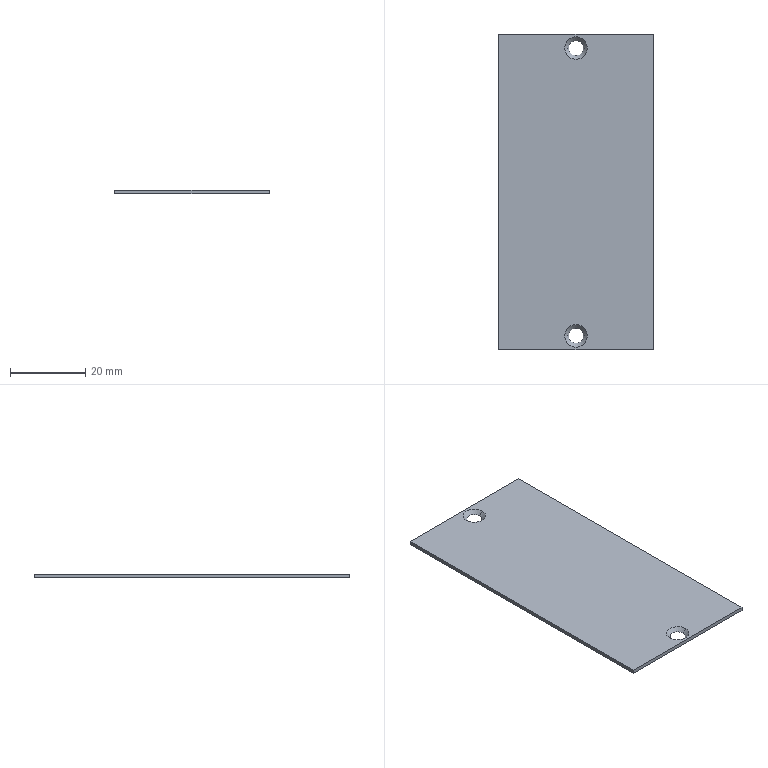Part | SolidWorks | features BaseBody 1 | 1 solid | 10 faces | box 41 x 84 x 1 mm | volume 3404 mm3 | plane 6 | cone 4
STEP:
#1=CARTESIAN_POINT('',(2.,-38.3,0.));
#2=VERTEX_POINT('',#1);
#3=CARTESIAN_POINT('',(-2.,-38.3,0.));
#4=VERTEX_POINT('',#3);
#5=CARTESIAN_POINT('',(0.,-38.3,0.));
#6=DIRECTION('',(0.,0.,-1.));
#7=DIRECTION('',(1.,0.,0.));
#8=AXIS2_PLACEMENT_3D('',#5,#6,#7);
#9=CIRCLE('',#8,2.);
#10=EDGE_CURVE('',#2,#4,#9,.T.);
#11=ORIENTED_EDGE('',*,*,#10,.T.);
#12=CARTESIAN_POINT('',(-3.,-38.3,1.));
#13=VERTEX_POINT('',#12);
#14=CARTESIAN_POINT('',(-3.,-38.3,1.));
#15=DIRECTION('',(-0.7071,0.,0.7071));
#16=VECTOR('',#15,1000.);
#17=LINE('',#14,#16);
#18=EDGE_CURVE('',#4,#13,#17,.T.);
#19=ORIENTED_EDGE('',*,*,#18,.T.);
#20=CARTESIAN_POINT('',(3.,-38.3,1.));
#21=VERTEX_POINT('',#20);
#22=CARTESIAN_POINT('',(0.,-38.3,1.));
#23=DIRECTION('',(0.,0.,-1.));
#24=DIRECTION('',(1.,0.,0.));
#25=AXIS2_PLACEMENT_3D('',#22,#23,#24);
#26=CIRCLE('',#25,3.);
#27=EDGE_CURVE('',#21,#13,#26,.T.);
#28=ORIENTED_EDGE('',*,*,#27,.F.);
#29=CARTESIAN_POINT('',(3.,-38.3,1.));
#30=DIRECTION('',(0.7071,0.,0.7071));
#31=VECTOR('',#30,1000.);
#32=LINE('',#29,#31);
#33=EDGE_CURVE('',#2,#21,#32,.T.);
#34=ORIENTED_EDGE('',*,*,#33,.F.);
#35=EDGE_LOOP('',(#11,#19,#28,#34));
#36=FACE_OUTER_BOUND('',#35,.T.);
#37=CARTESIAN_POINT('',(0.,-38.3,1.));
#38=DIRECTION('',(0.,0.,1.));
#39=DIRECTION('',(1.,0.,0.));
#40=AXIS2_PLACEMENT_3D('',#37,#38,#39);
#41=CONICAL_SURFACE('',#40,3.,0.7854);
#42=ADVANCED_FACE('',(#36),#41,.F.);
#43=CARTESIAN_POINT('',(2.,38.3,0.));
#44=VERTEX_POINT('',#43);
#45=CARTESIAN_POINT('',(-2.,38.3,0.));
#46=VERTEX_POINT('',#45);
#47=CARTESIAN_POINT('',(0.,38.3,0.));
#48=DIRECTION('',(0.,0.,-1.));
#49=DIRECTION('',(1.,0.,0.));
#50=AXIS2_PLACEMENT_3D('',#47,#48,#49);
#51=CIRCLE('',#50,2.);
#52=EDGE_CURVE('',#44,#46,#51,.T.);
#53=ORIENTED_EDGE('',*,*,#52,.T.);
#54=CARTESIAN_POINT('',(-3.,38.3,1.));
#55=VERTEX_POINT('',#54);
#56=CARTESIAN_POINT('',(-3.,38.3,1.));
#57=DIRECTION('',(-0.7071,0.,0.7071));
#58=VECTOR('',#57,1000.);
#59=LINE('',#56,#58);
#60=EDGE_CURVE('',#46,#55,#59,.T.);
#61=ORIENTED_EDGE('',*,*,#60,.T.);
#62=CARTESIAN_POINT('',(3.,38.3,1.));
#63=VERTEX_POINT('',#62);
#64=CARTESIAN_POINT('',(0.,38.3,1.));
#65=DIRECTION('',(0.,0.,-1.));
#66=DIRECTION('',(1.,0.,0.));
#67=AXIS2_PLACEMENT_3D('',#64,#65,#66);
#68=CIRCLE('',#67,3.);
#69=EDGE_CURVE('',#63,#55,#68,.T.);
#70=ORIENTED_EDGE('',*,*,#69,.F.);
#71=CARTESIAN_POINT('',(3.,38.3,1.));
#72=DIRECTION('',(0.7071,0.,0.7071));
#73=VECTOR('',#72,1000.);
#74=LINE('',#71,#73);
#75=EDGE_CURVE('',#44,#63,#74,.T.);
#76=ORIENTED_EDGE('',*,*,#75,.F.);
#77=EDGE_LOOP('',(#53,#61,#70,#76));
#78=FACE_OUTER_BOUND('',#77,.T.);
#79=CARTESIAN_POINT('',(0.,38.3,1.));
#80=DIRECTION('',(0.,0.,1.));
#81=DIRECTION('',(1.,0.,0.));
#82=AXIS2_PLACEMENT_3D('',#79,#80,#81);
#83=CONICAL_SURFACE('',#82,3.,0.7854);
#84=ADVANCED_FACE('',(#78),#83,.F.);
#85=ORIENTED_EDGE('',*,*,#10,.F.);
#86=CARTESIAN_POINT('',(0.,-38.3,0.));
#87=DIRECTION('',(0.,0.,-1.));
#88=DIRECTION('',(1.,0.,0.));
#89=AXIS2_PLACEMENT_3D('',#86,#87,#88);
#90=CIRCLE('',#89,2.);
#91=EDGE_CURVE('',#4,#2,#90,.T.);
#92=ORIENTED_EDGE('',*,*,#91,.F.);
#93=EDGE_LOOP('',(#85,#92));
#94=FACE_BOUND('',#93,.T.);
#95=ORIENTED_EDGE('',*,*,#52,.F.);
#96=CARTESIAN_POINT('',(0.,38.3,0.));
#97=DIRECTION('',(0.,0.,-1.));
#98=DIRECTION('',(1.,0.,0.));
#99=AXIS2_PLACEMENT_3D('',#96,#97,#98);
#100=CIRCLE('',#99,2.);
#101=EDGE_CURVE('',#46,#44,#100,.T.);
#102=ORIENTED_EDGE('',*,*,#101,.F.);
#103=EDGE_LOOP('',(#95,#102));
#104=FACE_BOUND('',#103,.T.);
#105=CARTESIAN_POINT('',(20.5,-42.,0.));
#106=VERTEX_POINT('',#105);
#107=CARTESIAN_POINT('',(20.5,42.,0.));
#108=VERTEX_POINT('',#107);
#109=CARTESIAN_POINT('',(20.5,0.,0.));
#110=DIRECTION('',(0.,1.,0.));
#111=VECTOR('',#110,1000.);
#112=LINE('',#109,#111);
#113=EDGE_CURVE('',#106,#108,#112,.T.);
#114=ORIENTED_EDGE('',*,*,#113,.F.);
#115=CARTESIAN_POINT('',(-20.5,-42.,0.));
#116=VERTEX_POINT('',#115);
#117=CARTESIAN_POINT('',(0.,-42.,0.));
#118=DIRECTION('',(1.,0.,0.));
#119=VECTOR('',#118,1000.);
#120=LINE('',#117,#119);
#121=EDGE_CURVE('',#116,#106,#120,.T.);
#122=ORIENTED_EDGE('',*,*,#121,.F.);
#123=CARTESIAN_POINT('',(-20.5,42.,0.));
#124=VERTEX_POINT('',#123);
#125=CARTESIAN_POINT('',(-20.5,0.,0.));
#126=DIRECTION('',(0.,-1.,0.));
#127=VECTOR('',#126,1000.);
#128=LINE('',#125,#127);
#129=EDGE_CURVE('',#124,#116,#128,.T.);
#130=ORIENTED_EDGE('',*,*,#129,.F.);
#131=CARTESIAN_POINT('',(0.,42.,0.));
#132=DIRECTION('',(-1.,0.,0.));
#133=VECTOR('',#132,1000.);
#134=LINE('',#131,#133);
#135=EDGE_CURVE('',#108,#124,#134,.T.);
#136=ORIENTED_EDGE('',*,*,#135,.F.);
#137=EDGE_LOOP('',(#114,#122,#130,#136));
#138=FACE_OUTER_BOUND('',#137,.T.);
#139=CARTESIAN_POINT('',(0.,0.,0.));
#140=DIRECTION('',(0.,0.,1.));
#141=DIRECTION('',(1.,0.,0.));
#142=AXIS2_PLACEMENT_3D('',#139,#140,#141);
#143=PLANE('',#142);
#144=ADVANCED_FACE('',(#94,#104,#138),#143,.F.);
#145=ORIENTED_EDGE('',*,*,#18,.F.);
#146=ORIENTED_EDGE('',*,*,#91,.T.);
#147=ORIENTED_EDGE('',*,*,#33,.T.);
#148=CARTESIAN_POINT('',(0.,-38.3,1.));
#149=DIRECTION('',(0.,0.,-1.));
#150=DIRECTION('',(1.,0.,0.));
#151=AXIS2_PLACEMENT_3D('',#148,#149,#150);
#152=CIRCLE('',#151,3.);
#153=EDGE_CURVE('',#13,#21,#152,.T.);
#154=ORIENTED_EDGE('',*,*,#153,.F.);
#155=EDGE_LOOP('',(#145,#146,#147,#154));
#156=FACE_OUTER_BOUND('',#155,.T.);
#157=CARTESIAN_POINT('',(0.,-38.3,1.));
#158=DIRECTION('',(0.,0.,1.));
#159=DIRECTION('',(1.,0.,0.));
#160=AXIS2_PLACEMENT_3D('',#157,#158,#159);
#161=CONICAL_SURFACE('',#160,3.,0.7854);
#162=ADVANCED_FACE('',(#156),#161,.F.);
#163=ORIENTED_EDGE('',*,*,#60,.F.);
#164=ORIENTED_EDGE('',*,*,#101,.T.);
#165=ORIENTED_EDGE('',*,*,#75,.T.);
#166=CARTESIAN_POINT('',(0.,38.3,1.));
#167=DIRECTION('',(0.,0.,-1.));
#168=DIRECTION('',(1.,0.,0.));
#169=AXIS2_PLACEMENT_3D('',#166,#167,#168);
#170=CIRCLE('',#169,3.);
#171=EDGE_CURVE('',#55,#63,#170,.T.);
#172=ORIENTED_EDGE('',*,*,#171,.F.);
#173=EDGE_LOOP('',(#163,#164,#165,#172));
#174=FACE_OUTER_BOUND('',#173,.T.);
#175=CARTESIAN_POINT('',(0.,38.3,1.));
#176=DIRECTION('',(0.,0.,1.));
#177=DIRECTION('',(1.,0.,0.));
#178=AXIS2_PLACEMENT_3D('',#175,#176,#177);
#179=CONICAL_SURFACE('',#178,3.,0.7854);
#180=ADVANCED_FACE('',(#174),#179,.F.);
#181=CARTESIAN_POINT('',(20.5,42.,1.));
#182=VERTEX_POINT('',#181);
#183=CARTESIAN_POINT('',(-20.5,42.,1.));
#184=VERTEX_POINT('',#183);
#185=CARTESIAN_POINT('',(0.,42.,1.));
#186=DIRECTION('',(-1.,0.,0.));
#187=VECTOR('',#186,1000.);
#188=LINE('',#185,#187);
#189=EDGE_CURVE('',#182,#184,#188,.T.);
#190=ORIENTED_EDGE('',*,*,#189,.F.);
#191=CARTESIAN_POINT('',(20.5,42.,0.5));
#192=DIRECTION('',(0.,0.,1.));
#193=VECTOR('',#192,1000.);
#194=LINE('',#191,#193);
#195=EDGE_CURVE('',#108,#182,#194,.T.);
#196=ORIENTED_EDGE('',*,*,#195,.F.);
#197=ORIENTED_EDGE('',*,*,#135,.T.);
#198=CARTESIAN_POINT('',(-20.5,42.,0.5));
#199=DIRECTION('',(0.,0.,-1.));
#200=VECTOR('',#199,1000.);
#201=LINE('',#198,#200);
#202=EDGE_CURVE('',#184,#124,#201,.T.);
#203=ORIENTED_EDGE('',*,*,#202,.F.);
#204=EDGE_LOOP('',(#190,#196,#197,#203));
#205=FACE_OUTER_BOUND('',#204,.T.);
#206=CARTESIAN_POINT('',(0.,42.,0.5));
#207=DIRECTION('',(0.,-1.,0.));
#208=DIRECTION('',(0.,0.,-1.));
#209=AXIS2_PLACEMENT_3D('',#206,#207,#208);
#210=PLANE('',#209);
#211=ADVANCED_FACE('',(#205),#210,.F.);
#212=CARTESIAN_POINT('',(20.5,-42.,1.));
#213=VERTEX_POINT('',#212);
#214=CARTESIAN_POINT('',(20.5,0.,1.));
#215=DIRECTION('',(0.,1.,0.));
#216=VECTOR('',#215,1000.);
#217=LINE('',#214,#216);
#218=EDGE_CURVE('',#213,#182,#217,.T.);
#219=ORIENTED_EDGE('',*,*,#218,.F.);
#220=CARTESIAN_POINT('',(20.5,-42.,0.5));
#221=DIRECTION('',(0.,0.,1.));
#222=VECTOR('',#221,1000.);
#223=LINE('',#220,#222);
#224=EDGE_CURVE('',#106,#213,#223,.T.);
#225=ORIENTED_EDGE('',*,*,#224,.F.);
#226=ORIENTED_EDGE('',*,*,#113,.T.);
#227=ORIENTED_EDGE('',*,*,#195,.T.);
#228=EDGE_LOOP('',(#219,#225,#226,#227));
#229=FACE_OUTER_BOUND('',#228,.T.);
#230=CARTESIAN_POINT('',(20.5,0.,0.5));
#231=DIRECTION('',(-1.,0.,0.));
#232=DIRECTION('',(0.,0.,1.));
#233=AXIS2_PLACEMENT_3D('',#230,#231,#232);
#234=PLANE('',#233);
#235=ADVANCED_FACE('',(#229),#234,.F.);
#236=CARTESIAN_POINT('',(-20.5,-42.,1.));
#237=VERTEX_POINT('',#236);
#238=CARTESIAN_POINT('',(0.,-42.,1.));
#239=DIRECTION('',(1.,0.,0.));
#240=VECTOR('',#239,1000.);
#241=LINE('',#238,#240);
#242=EDGE_CURVE('',#237,#213,#241,.T.);
#243=ORIENTED_EDGE('',*,*,#242,.F.);
#244=CARTESIAN_POINT('',(-20.5,-42.,0.5));
#245=DIRECTION('',(0.,0.,1.));
#246=VECTOR('',#245,1000.);
#247=LINE('',#244,#246);
#248=EDGE_CURVE('',#116,#237,#247,.T.);
#249=ORIENTED_EDGE('',*,*,#248,.F.);
#250=ORIENTED_EDGE('',*,*,#121,.T.);
#251=ORIENTED_EDGE('',*,*,#224,.T.);
#252=EDGE_LOOP('',(#243,#249,#250,#251));
#253=FACE_OUTER_BOUND('',#252,.T.);
#254=CARTESIAN_POINT('',(0.,-42.,0.5));
#255=DIRECTION('',(0.,1.,0.));
#256=DIRECTION('',(0.,0.,1.));
#257=AXIS2_PLACEMENT_3D('',#254,#255,#256);
#258=PLANE('',#257);
#259=ADVANCED_FACE('',(#253),#258,.F.);
#260=CARTESIAN_POINT('',(-20.5,0.,1.));
#261=DIRECTION('',(0.,-1.,0.));
#262=VECTOR('',#261,1000.);
#263=LINE('',#260,#262);
#264=EDGE_CURVE('',#184,#237,#263,.T.);
#265=ORIENTED_EDGE('',*,*,#264,.F.);
#266=ORIENTED_EDGE('',*,*,#202,.T.);
#267=ORIENTED_EDGE('',*,*,#129,.T.);
#268=ORIENTED_EDGE('',*,*,#248,.T.);
#269=EDGE_LOOP('',(#265,#266,#267,#268));
#270=FACE_OUTER_BOUND('',#269,.T.);
#271=CARTESIAN_POINT('',(-20.5,0.,0.5));
#272=DIRECTION('',(1.,0.,0.));
#273=DIRECTION('',(0.,0.,-1.));
#274=AXIS2_PLACEMENT_3D('',#271,#272,#273);
#275=PLANE('',#274);
#276=ADVANCED_FACE('',(#270),#275,.F.);
#277=ORIENTED_EDGE('',*,*,#27,.T.);
#278=ORIENTED_EDGE('',*,*,#153,.T.);
#279=EDGE_LOOP('',(#277,#278));
#280=FACE_BOUND('',#279,.T.);
#281=ORIENTED_EDGE('',*,*,#69,.T.);
#282=ORIENTED_EDGE('',*,*,#171,.T.);
#283=EDGE_LOOP('',(#281,#282));
#284=FACE_BOUND('',#283,.T.);
#285=ORIENTED_EDGE('',*,*,#189,.T.);
#286=ORIENTED_EDGE('',*,*,#264,.T.);
#287=ORIENTED_EDGE('',*,*,#242,.T.);
#288=ORIENTED_EDGE('',*,*,#218,.T.);
#289=EDGE_LOOP('',(#285,#286,#287,#288));
#290=FACE_OUTER_BOUND('',#289,.T.);
#291=CARTESIAN_POINT('',(0.,0.,1.));
#292=DIRECTION('',(0.,0.,1.));
#293=DIRECTION('',(1.,0.,0.));
#294=AXIS2_PLACEMENT_3D('',#291,#292,#293);
#295=PLANE('',#294);
#296=ADVANCED_FACE('',(#280,#284,#290),#295,.T.);
#297=CLOSED_SHELL('',(#42,#84,#144,#162,#180,#211,#235,#259,#276,#296));
#298=MANIFOLD_SOLID_BREP('',#297);
#299=CARTESIAN_POINT('',(0.,0.,0.));
#300=DIRECTION('',(0.,0.,1.));
#301=DIRECTION('',(1.,0.,0.));
#302=AXIS2_PLACEMENT_3D('',#299,#300,#301);
#303=(LENGTH_UNIT()NAMED_UNIT(*)SI_UNIT(.MILLI.,.METRE.));
#304=UNCERTAINTY_MEASURE_WITH_UNIT(LENGTH_MEASURE(0.00001),#303,'','');
#305=(NAMED_UNIT(*)PLANE_ANGLE_UNIT()SI_UNIT($,.RADIAN.));
#306=(NAMED_UNIT(*)SI_UNIT($,.STERADIAN.)SOLID_ANGLE_UNIT());
#307=(GEOMETRIC_REPRESENTATION_CONTEXT(3)GLOBAL_UNCERTAINTY_ASSIGNED_CONTEXT((#304))GLOBAL_UNIT_ASSIGNED_CONTEXT((#303,#305,#306))REPRESENTATION_CONTEXT('',''));
#308=ADVANCED_BREP_SHAPE_REPRESENTATION('',(#298,#302),#307);